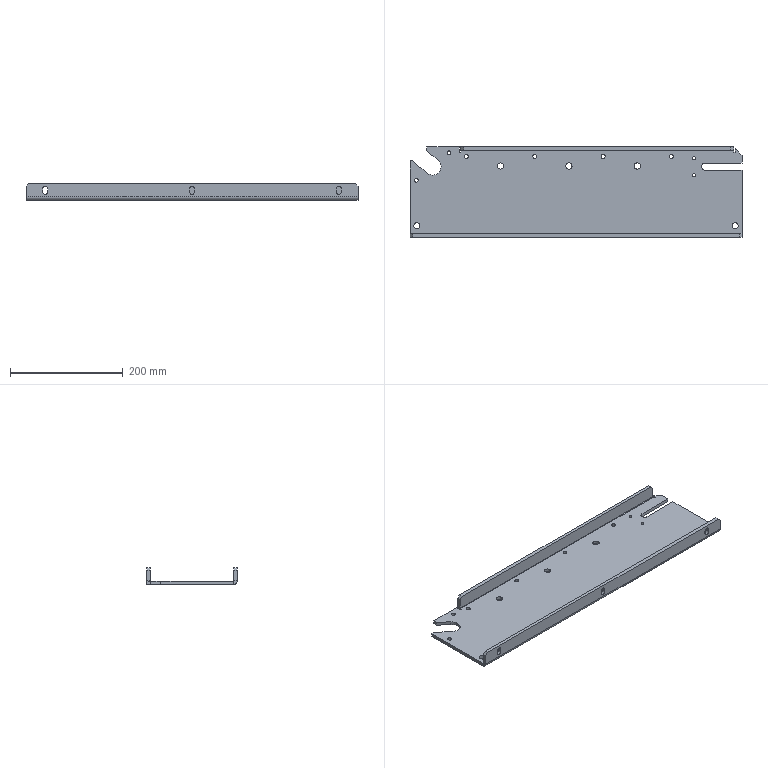Part | SolidWorks | features BaseBody 1 | 1 solid | 85 faces | box 588 x 160 x 30 mm | volume 684880 mm3 | plane 43 | cylinder 42 | commonest cylinder face diameters 11 x10 9 x9 7 x8 5 x4 6.8 x4 1.473 x2